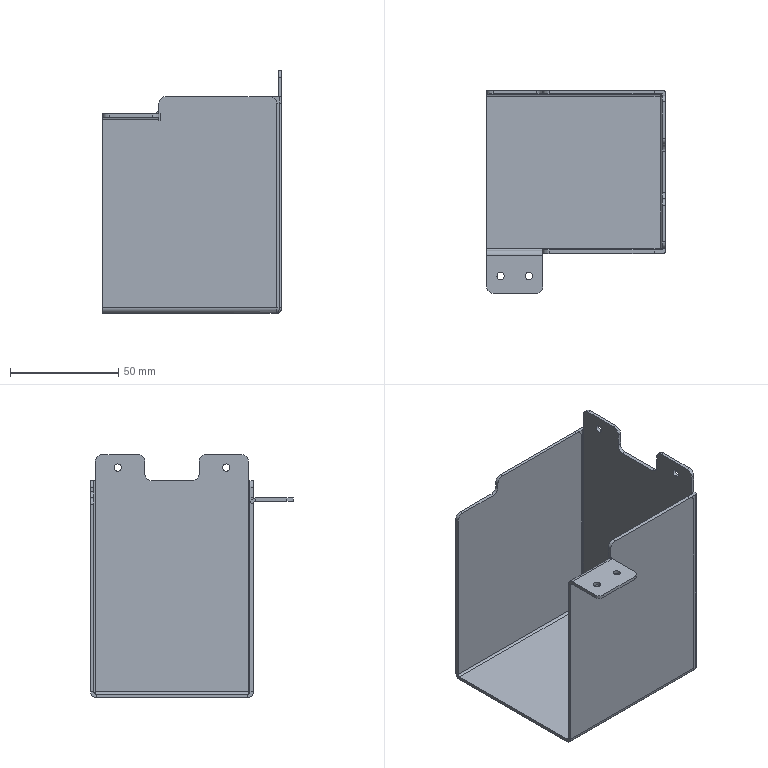Part | SolidWorks | features EdgeFlange 2, HoleWzd 2, ICE 2, SMWeldBead 2, BreakCorner 1, FlatPattern 1, MoveFace 1, SMBaseFlange 1, SheetMetal 1 | 1 solid | 92 faces | box 82.5 x 93.5 x 112 mm | volume 44800 mm3 | plane 50 | cylinder 32 | spline 10 | commonest cylinder face diameters 6 x12 2 x8 3.4 x8 5 x4